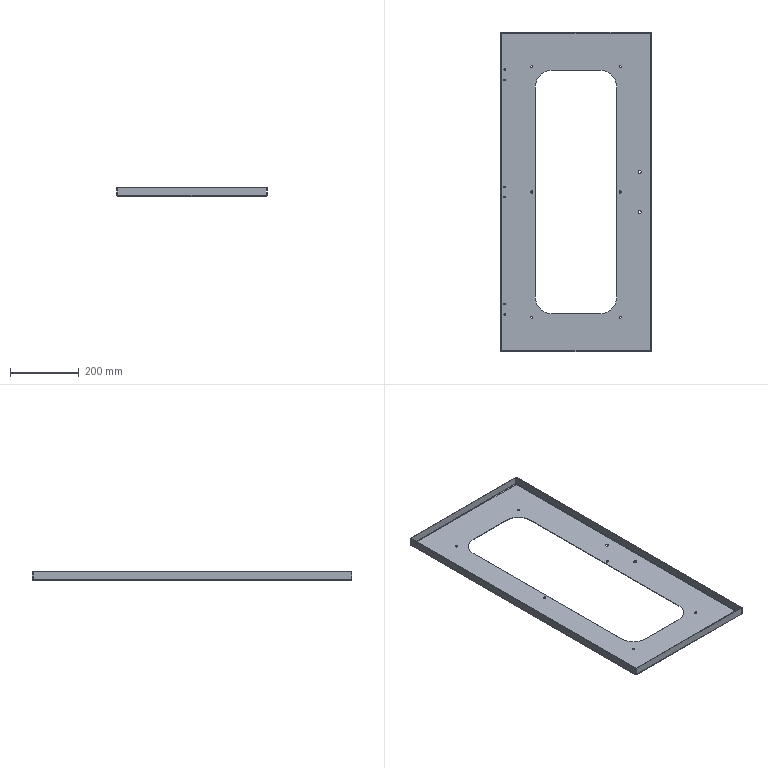Part | STEP file | SynoNew-0304-060 | 1 solid | 64 faces | box 437 x 930 x 25 mm | volume 451749 mm3 | plane 38 | cylinder 26 | commonest cylinder face diameters 4.2 x6 6.6 x6 3 x4 6 x4 100 x4 9 x2